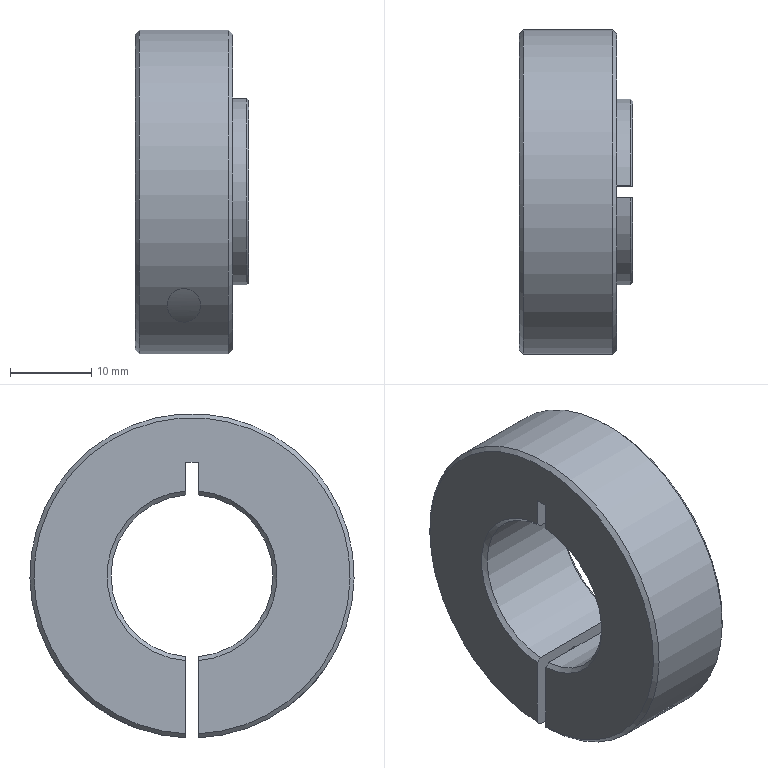Part | NX | features 1_11 2 | 1 solid | 28 faces | box 14 x 40 x 39.986 mm | volume 10434 mm3 | plane 10 | cone 9 | cylinder 9 | commonest cylinder face diameters 20 x2 23 x2 40 x2 4.134 x1 5.5 x1 9 x1
STEP:
#1=CARTESIAN_POINT('',(-123.,-261.55,-709.529));
#2=VERTEX_POINT('',#1);
#3=CARTESIAN_POINT('',(-125.5,-261.55,-709.529));
#4=DIRECTION('',(0.,-1.,0.));
#5=DIRECTION('',(1.,0.,0.));
#6=AXIS2_PLACEMENT_3D('',#3,#4,#5);
#7=CIRCLE('',#6,2.5);
#8=EDGE_CURVE('',#2,#2,#7,.T.);
#9=ORIENTED_EDGE('',*,*,#8,.F.);
#10=EDGE_LOOP('',(#9));
#11=FACE_BOUND('',#10,.T.);
#12=CARTESIAN_POINT('',(-127.567,-261.983,-709.529));
#13=VERTEX_POINT('',#12);
#14=CARTESIAN_POINT('',(-125.5,-261.983,-709.529));
#15=DIRECTION('',(0.,-1.,0.));
#16=DIRECTION('',(-1.,0.,0.));
#17=AXIS2_PLACEMENT_3D('',#14,#15,#16);
#18=CIRCLE('',#17,2.067);
#19=EDGE_CURVE('',#13,#13,#18,.T.);
#20=ORIENTED_EDGE('',*,*,#19,.T.);
#21=EDGE_LOOP('',(#20));
#22=FACE_BOUND('',#21,.T.);
#23=CARTESIAN_POINT('',(-125.5,-262.032,-709.529));
#24=DIRECTION('',(0.,1.,0.));
#25=DIRECTION('',(-1.,0.,0.));
#26=AXIS2_PLACEMENT_3D('',#23,#24,#25);
#27=CONICAL_SURFACE('',#26,2.018,0.7854);
#28=ADVANCED_FACE('',(#11,#22),#27,.F.);
#29=CARTESIAN_POINT('',(-127.567,-275.083,-709.529));
#30=VERTEX_POINT('',#29);
#31=CARTESIAN_POINT('',(-123.433,-275.083,-709.529));
#32=VERTEX_POINT('',#31);
#33=CARTESIAN_POINT('',(-123.433,-275.083,-709.529));
#34=CARTESIAN_POINT('',(-123.433,-274.603,-710.02));
#35=CARTESIAN_POINT('',(-123.683,-273.842,-710.714));
#36=CARTESIAN_POINT('',(-124.497,-272.96,-711.413));
#37=CARTESIAN_POINT('',(-125.5,-272.586,-711.688));
#38=CARTESIAN_POINT('',(-126.503,-272.96,-711.413));
#39=CARTESIAN_POINT('',(-127.317,-273.842,-710.714));
#40=CARTESIAN_POINT('',(-127.567,-274.603,-710.02));
#41=CARTESIAN_POINT('',(-127.567,-275.083,-709.529));
#42=B_SPLINE_CURVE_WITH_KNOTS('',3,(#33,#34,#35,#36,#37,#38,#39,#40,#41),.UNSPECIFIED.,.F.,.F.,(4,1,1,1,1,1,4),(0.,0.25,0.375,0.5,0.625,0.75,1.),.UNSPECIFIED.);
#43=EDGE_CURVE('',#30,#32,#42,.F.);
#44=ORIENTED_EDGE('',*,*,#43,.T.);
#45=CARTESIAN_POINT('',(-127.567,-275.083,-709.529));
#46=CARTESIAN_POINT('',(-127.567,-275.524,-709.078));
#47=CARTESIAN_POINT('',(-127.348,-276.166,-708.351));
#48=CARTESIAN_POINT('',(-126.445,-276.738,-707.615));
#49=CARTESIAN_POINT('',(-125.5,-276.906,-707.386));
#50=CARTESIAN_POINT('',(-124.555,-276.738,-707.615));
#51=CARTESIAN_POINT('',(-123.652,-276.166,-708.351));
#52=CARTESIAN_POINT('',(-123.433,-275.524,-709.078));
#53=CARTESIAN_POINT('',(-123.433,-275.083,-709.529));
#54=B_SPLINE_CURVE_WITH_KNOTS('',3,(#45,#46,#47,#48,#49,#50,#51,#52,#53),.UNSPECIFIED.,.F.,.F.,(4,1,1,1,1,1,4),(0.,0.25,0.375,0.5,0.625,0.75,1.),.UNSPECIFIED.);
#55=EDGE_CURVE('',#32,#30,#54,.F.);
#56=ORIENTED_EDGE('',*,*,#55,.T.);
#57=EDGE_LOOP('',(#44,#56));
#58=FACE_BOUND('',#57,.T.);
#59=ORIENTED_EDGE('',*,*,#19,.F.);
#60=EDGE_LOOP('',(#59));
#61=FACE_BOUND('',#60,.T.);
#62=CARTESIAN_POINT('',(-125.5,-272.267,-709.529));
#63=DIRECTION('',(0.,-1.,0.));
#64=DIRECTION('',(1.,0.,0.));
#65=AXIS2_PLACEMENT_3D('',#62,#63,#64);
#66=CYLINDRICAL_SURFACE('',#65,2.067);
#67=ADVANCED_FACE('',(#58,#61),#66,.F.);
#68=CARTESIAN_POINT('',(-131.5,-261.55,-681.529));
#69=VERTEX_POINT('',#68);
#70=CARTESIAN_POINT('',(-131.5,-260.05,-681.529));
#71=VERTEX_POINT('',#70);
#72=CARTESIAN_POINT('',(-131.5,-261.55,-681.529));
#73=DIRECTION('',(0.,1.,0.));
#74=VECTOR('',#73,1000.);
#75=LINE('',#72,#74);
#76=EDGE_CURVE('',#69,#71,#75,.T.);
#77=ORIENTED_EDGE('',*,*,#76,.T.);
#78=CARTESIAN_POINT('',(-119.5,-260.05,-681.529));
#79=VERTEX_POINT('',#78);
#80=CARTESIAN_POINT('',(-119.5,-260.05,-681.529));
#81=DIRECTION('',(-1.,0.,0.));
#82=VECTOR('',#81,1000.);
#83=LINE('',#80,#82);
#84=EDGE_CURVE('',#79,#71,#83,.T.);
#85=ORIENTED_EDGE('',*,*,#84,.F.);
#86=CARTESIAN_POINT('',(-119.5,-261.55,-681.529));
#87=VERTEX_POINT('',#86);
#88=CARTESIAN_POINT('',(-119.5,-260.05,-681.529));
#89=DIRECTION('',(0.,-1.,0.));
#90=VECTOR('',#89,1000.);
#91=LINE('',#88,#90);
#92=EDGE_CURVE('',#79,#87,#91,.T.);
#93=ORIENTED_EDGE('',*,*,#92,.T.);
#94=CARTESIAN_POINT('',(-131.5,-261.55,-681.529));
#95=DIRECTION('',(1.,0.,0.));
#96=VECTOR('',#95,1000.);
#97=LINE('',#94,#96);
#98=EDGE_CURVE('',#69,#87,#97,.T.);
#99=ORIENTED_EDGE('',*,*,#98,.F.);
#100=EDGE_LOOP('',(#77,#85,#93,#99));
#101=FACE_BOUND('',#100,.T.);
#102=CARTESIAN_POINT('',(-149.5,-261.55,-681.529));
#103=DIRECTION('',(0.,0.,1.));
#104=DIRECTION('',(0.,1.,0.));
#105=AXIS2_PLACEMENT_3D('',#102,#103,#104);
#106=PLANE('',#105);
#107=ADVANCED_FACE('',(#101),#106,.F.);
#108=CARTESIAN_POINT('',(-131.5,-260.05,-685.056));
#109=VERTEX_POINT('',#108);
#110=CARTESIAN_POINT('',(-131.5,-260.05,-681.529));
#111=DIRECTION('',(0.,0.,-1.));
#112=VECTOR('',#111,1000.);
#113=LINE('',#110,#112);
#114=EDGE_CURVE('',#71,#109,#113,.T.);
#115=ORIENTED_EDGE('',*,*,#114,.T.);
#116=CARTESIAN_POINT('',(-131.,-260.05,-685.558));
#117=VERTEX_POINT('',#116);
#118=CARTESIAN_POINT('',(-131.5,-260.05,-685.056));
#119=CARTESIAN_POINT('',(-131.333,-260.05,-685.223));
#120=CARTESIAN_POINT('',(-131.167,-260.05,-685.39));
#121=CARTESIAN_POINT('',(-131.,-260.05,-685.558));
#122=B_SPLINE_CURVE_WITH_KNOTS('',3,(#118,#119,#120,#121),.UNSPECIFIED.,.F.,.F.,(4,4),(0.,1.),.UNSPECIFIED.);
#123=EDGE_CURVE('',#117,#109,#122,.F.);
#124=ORIENTED_EDGE('',*,*,#123,.F.);
#125=CARTESIAN_POINT('',(-118.,-260.05,-685.558));
#126=VERTEX_POINT('',#125);
#127=CARTESIAN_POINT('',(-118.,-260.05,-685.558));
#128=DIRECTION('',(-1.,0.,0.));
#129=VECTOR('',#128,1000.);
#130=LINE('',#127,#129);
#131=EDGE_CURVE('',#126,#117,#130,.T.);
#132=ORIENTED_EDGE('',*,*,#131,.F.);
#133=CARTESIAN_POINT('',(-117.5,-260.05,-685.056));
#134=VERTEX_POINT('',#133);
#135=CARTESIAN_POINT('',(-118.,-260.05,-685.558));
#136=CARTESIAN_POINT('',(-117.833,-260.05,-685.39));
#137=CARTESIAN_POINT('',(-117.667,-260.05,-685.223));
#138=CARTESIAN_POINT('',(-117.5,-260.05,-685.056));
#139=B_SPLINE_CURVE_WITH_KNOTS('',3,(#135,#136,#137,#138),.UNSPECIFIED.,.F.,.F.,(4,4),(0.,1.),.UNSPECIFIED.);
#140=EDGE_CURVE('',#134,#126,#139,.F.);
#141=ORIENTED_EDGE('',*,*,#140,.F.);
#142=CARTESIAN_POINT('',(-117.5,-260.05,-684.279));
#143=VERTEX_POINT('',#142);
#144=CARTESIAN_POINT('',(-117.5,-260.05,-685.056));
#145=DIRECTION('',(0.,0.,1.));
#146=VECTOR('',#145,1000.);
#147=LINE('',#144,#146);
#148=EDGE_CURVE('',#134,#143,#147,.T.);
#149=ORIENTED_EDGE('',*,*,#148,.T.);
#150=CARTESIAN_POINT('',(-117.725,-260.05,-684.054));
#151=VERTEX_POINT('',#150);
#152=CARTESIAN_POINT('',(-117.5,-260.05,-684.279));
#153=CARTESIAN_POINT('',(-117.575,-260.05,-684.204));
#154=CARTESIAN_POINT('',(-117.65,-260.05,-684.129));
#155=CARTESIAN_POINT('',(-117.725,-260.05,-684.054));
#156=B_SPLINE_CURVE_WITH_KNOTS('',3,(#152,#153,#154,#155),.UNSPECIFIED.,.F.,.F.,(4,4),(0.,1.),.UNSPECIFIED.);
#157=EDGE_CURVE('',#151,#143,#156,.F.);
#158=ORIENTED_EDGE('',*,*,#157,.F.);
#159=CARTESIAN_POINT('',(-119.5,-260.05,-684.054));
#160=VERTEX_POINT('',#159);
#161=CARTESIAN_POINT('',(-119.5,-260.05,-684.054));
#162=DIRECTION('',(1.,0.,0.));
#163=VECTOR('',#162,1000.);
#164=LINE('',#161,#163);
#165=EDGE_CURVE('',#160,#151,#164,.T.);
#166=ORIENTED_EDGE('',*,*,#165,.F.);
#167=CARTESIAN_POINT('',(-119.5,-260.05,-684.054));
#168=DIRECTION('',(0.,0.,1.));
#169=VECTOR('',#168,1000.);
#170=LINE('',#167,#169);
#171=EDGE_CURVE('',#160,#79,#170,.T.);
#172=ORIENTED_EDGE('',*,*,#171,.T.);
#173=ORIENTED_EDGE('',*,*,#84,.T.);
#174=EDGE_LOOP('',(#115,#124,#132,#141,#149,#158,#166,#172,#173));
#175=FACE_BOUND('',#174,.T.);
#176=CARTESIAN_POINT('',(-149.5,-260.05,-681.529));
#177=DIRECTION('',(0.,1.,0.));
#178=DIRECTION('',(-1.,0.,0.));
#179=AXIS2_PLACEMENT_3D('',#176,#177,#178);
#180=PLANE('',#179);
#181=ADVANCED_FACE('',(#175),#180,.F.);
#182=CARTESIAN_POINT('',(-131.,-260.05,-705.501));
#183=VERTEX_POINT('',#182);
#184=CARTESIAN_POINT('',(-131.,-260.8,-695.529));
#185=DIRECTION('',(1.,0.,0.));
#186=DIRECTION('',(0.,1.,0.));
#187=AXIS2_PLACEMENT_3D('',#184,#185,#186);
#188=CIRCLE('',#187,10.);
#189=EDGE_CURVE('',#183,#117,#188,.T.);
#190=ORIENTED_EDGE('',*,*,#189,.F.);
#191=CARTESIAN_POINT('',(-118.,-260.05,-705.501));
#192=VERTEX_POINT('',#191);
#193=CARTESIAN_POINT('',(-131.,-260.05,-705.501));
#194=DIRECTION('',(1.,0.,0.));
#195=VECTOR('',#194,1000.);
#196=LINE('',#193,#195);
#197=EDGE_CURVE('',#183,#192,#196,.T.);
#198=ORIENTED_EDGE('',*,*,#197,.T.);
#199=CARTESIAN_POINT('',(-118.,-260.8,-695.529));
#200=DIRECTION('',(-1.,0.,0.));
#201=DIRECTION('',(0.,1.,0.));
#202=AXIS2_PLACEMENT_3D('',#199,#200,#201);
#203=CIRCLE('',#202,10.);
#204=EDGE_CURVE('',#126,#192,#203,.T.);
#205=ORIENTED_EDGE('',*,*,#204,.F.);
#206=ORIENTED_EDGE('',*,*,#131,.T.);
#207=EDGE_LOOP('',(#190,#198,#205,#206));
#208=FACE_BOUND('',#207,.T.);
#209=CARTESIAN_POINT('',(-124.5,-260.8,-695.529));
#210=DIRECTION('',(-1.,0.,0.));
#211=DIRECTION('',(0.,-1.,0.));
#212=AXIS2_PLACEMENT_3D('',#209,#210,#211);
#213=CYLINDRICAL_SURFACE('',#212,10.);
#214=ADVANCED_FACE('',(#208),#213,.F.);
#215=ORIENTED_EDGE('',*,*,#204,.T.);
#216=CARTESIAN_POINT('',(-117.5,-260.05,-706.003));
#217=VERTEX_POINT('',#216);
#218=CARTESIAN_POINT('',(-117.5,-260.05,-706.003));
#219=CARTESIAN_POINT('',(-117.667,-260.05,-705.835));
#220=CARTESIAN_POINT('',(-117.833,-260.05,-705.668));
#221=CARTESIAN_POINT('',(-118.,-260.05,-705.501));
#222=B_SPLINE_CURVE_WITH_KNOTS('',3,(#218,#219,#220,#221),.UNSPECIFIED.,.F.,.F.,(4,4),(0.,1.),.UNSPECIFIED.);
#223=EDGE_CURVE('',#192,#217,#222,.F.);
#224=ORIENTED_EDGE('',*,*,#223,.T.);
#225=CARTESIAN_POINT('',(-117.5,-260.8,-695.529));
#226=DIRECTION('',(-1.,0.,0.));
#227=DIRECTION('',(0.,1.,0.));
#228=AXIS2_PLACEMENT_3D('',#225,#226,#227);
#229=CIRCLE('',#228,10.5);
#230=EDGE_CURVE('',#134,#217,#229,.T.);
#231=ORIENTED_EDGE('',*,*,#230,.F.);
#232=ORIENTED_EDGE('',*,*,#140,.T.);
#233=EDGE_LOOP('',(#215,#224,#231,#232));
#234=FACE_BOUND('',#233,.T.);
#235=CARTESIAN_POINT('',(-118.049,-260.8,-695.529));
#236=DIRECTION('',(1.,0.,0.));
#237=DIRECTION('',(0.,1.,0.));
#238=AXIS2_PLACEMENT_3D('',#235,#236,#237);
#239=CONICAL_SURFACE('',#238,9.951,0.7854);
#240=ADVANCED_FACE('',(#234),#239,.F.);
#241=CARTESIAN_POINT('',(-117.5,-260.05,-706.779));
#242=VERTEX_POINT('',#241);
#243=CARTESIAN_POINT('',(-117.5,-260.8,-695.529));
#244=DIRECTION('',(1.,0.,0.));
#245=DIRECTION('',(0.,0.06652,-0.9978));
#246=AXIS2_PLACEMENT_3D('',#243,#244,#245);
#247=CIRCLE('',#246,11.275);
#248=EDGE_CURVE('',#242,#143,#247,.T.);
#249=ORIENTED_EDGE('',*,*,#248,.T.);
#250=ORIENTED_EDGE('',*,*,#148,.F.);
#251=ORIENTED_EDGE('',*,*,#230,.T.);
#252=CARTESIAN_POINT('',(-117.5,-260.05,-706.779));
#253=DIRECTION('',(0.,0.,1.));
#254=VECTOR('',#253,1000.);
#255=LINE('',#252,#254);
#256=EDGE_CURVE('',#242,#217,#255,.T.);
#257=ORIENTED_EDGE('',*,*,#256,.F.);
#258=EDGE_LOOP('',(#249,#250,#251,#257));
#259=FACE_BOUND('',#258,.T.);
#260=CARTESIAN_POINT('',(-117.5,-260.8,-684.642));
#261=DIRECTION('',(1.,0.,0.));
#262=DIRECTION('',(0.,1.,0.));
#263=AXIS2_PLACEMENT_3D('',#260,#261,#262);
#264=PLANE('',#263);
#265=ADVANCED_FACE('',(#259),#264,.T.);
#266=CARTESIAN_POINT('',(-117.725,-260.05,-707.005));
#267=VERTEX_POINT('',#266);
#268=CARTESIAN_POINT('',(-117.725,-260.8,-695.529));
#269=DIRECTION('',(1.,0.,0.));
#270=DIRECTION('',(0.,0.06522,-0.9979));
#271=AXIS2_PLACEMENT_3D('',#268,#269,#270);
#272=CIRCLE('',#271,11.5);
#273=EDGE_CURVE('',#267,#151,#272,.T.);
#274=ORIENTED_EDGE('',*,*,#273,.T.);
#275=ORIENTED_EDGE('',*,*,#157,.T.);
#276=ORIENTED_EDGE('',*,*,#248,.F.);
#277=CARTESIAN_POINT('',(-117.725,-260.05,-707.005));
#278=CARTESIAN_POINT('',(-117.65,-260.05,-706.93));
#279=CARTESIAN_POINT('',(-117.575,-260.05,-706.855));
#280=CARTESIAN_POINT('',(-117.5,-260.05,-706.779));
#281=B_SPLINE_CURVE_WITH_KNOTS('',3,(#277,#278,#279,#280),.UNSPECIFIED.,.F.,.F.,(4,4),(0.,1.),.UNSPECIFIED.);
#282=EDGE_CURVE('',#242,#267,#281,.F.);
#283=ORIENTED_EDGE('',*,*,#282,.T.);
#284=EDGE_LOOP('',(#274,#275,#276,#283));
#285=FACE_BOUND('',#284,.T.);
#286=CARTESIAN_POINT('',(-117.451,-260.8,-695.529));
#287=DIRECTION('',(-1.,0.,0.));
#288=DIRECTION('',(0.,-1.,0.));
#289=AXIS2_PLACEMENT_3D('',#286,#287,#288);
#290=CONICAL_SURFACE('',#289,11.226,0.7854);
#291=ADVANCED_FACE('',(#285),#290,.T.);
#292=CARTESIAN_POINT('',(-119.5,-260.05,-707.005));
#293=VERTEX_POINT('',#292);
#294=CARTESIAN_POINT('',(-119.5,-260.8,-695.529));
#295=DIRECTION('',(-1.,0.,0.));
#296=DIRECTION('',(0.,1.,0.));
#297=AXIS2_PLACEMENT_3D('',#294,#295,#296);
#298=CIRCLE('',#297,11.5);
#299=EDGE_CURVE('',#160,#293,#298,.T.);
#300=ORIENTED_EDGE('',*,*,#299,.F.);
#301=ORIENTED_EDGE('',*,*,#165,.T.);
#302=ORIENTED_EDGE('',*,*,#273,.F.);
#303=CARTESIAN_POINT('',(-117.725,-260.05,-707.005));
#304=DIRECTION('',(-1.,0.,0.));
#305=VECTOR('',#304,1000.);
#306=LINE('',#303,#305);
#307=EDGE_CURVE('',#267,#293,#306,.T.);
#308=ORIENTED_EDGE('',*,*,#307,.T.);
#309=EDGE_LOOP('',(#300,#301,#302,#308));
#310=FACE_BOUND('',#309,.T.);
#311=CARTESIAN_POINT('',(-118.612,-260.8,-695.529));
#312=DIRECTION('',(-1.,0.,0.));
#313=DIRECTION('',(0.,-1.,0.));
#314=AXIS2_PLACEMENT_3D('',#311,#312,#313);
#315=CYLINDRICAL_SURFACE('',#314,11.5);
#316=ADVANCED_FACE('',(#310),#315,.T.);
#317=CARTESIAN_POINT('',(-119.5,-260.05,-715.015));
#318=VERTEX_POINT('',#317);
#319=CARTESIAN_POINT('',(-119.5,-260.05,-715.015));
#320=DIRECTION('',(0.,0.,1.));
#321=VECTOR('',#320,1000.);
#322=LINE('',#319,#321);
#323=EDGE_CURVE('',#318,#293,#322,.T.);
#324=ORIENTED_EDGE('',*,*,#323,.F.);
#325=CARTESIAN_POINT('',(-119.5,-261.55,-715.015));
#326=VERTEX_POINT('',#325);
#327=CARTESIAN_POINT('',(-119.5,-260.8,-695.529));
#328=DIRECTION('',(1.,0.,0.));
#329=DIRECTION('',(0.,1.,0.));
#330=AXIS2_PLACEMENT_3D('',#327,#328,#329);
#331=CIRCLE('',#330,19.5);
#332=EDGE_CURVE('',#318,#326,#331,.T.);
#333=ORIENTED_EDGE('',*,*,#332,.T.);
#334=CARTESIAN_POINT('',(-119.5,-261.55,-707.005));
#335=VERTEX_POINT('',#334);
#336=CARTESIAN_POINT('',(-119.5,-261.55,-707.005));
#337=DIRECTION('',(0.,0.,-1.));
#338=VECTOR('',#337,1000.);
#339=LINE('',#336,#338);
#340=EDGE_CURVE('',#335,#326,#339,.T.);
#341=ORIENTED_EDGE('',*,*,#340,.F.);
#342=CARTESIAN_POINT('',(-119.5,-261.55,-684.054));
#343=VERTEX_POINT('',#342);
#344=CARTESIAN_POINT('',(-119.5,-260.8,-695.529));
#345=DIRECTION('',(-1.,0.,0.));
#346=DIRECTION('',(0.,-1.,0.));
#347=AXIS2_PLACEMENT_3D('',#344,#345,#346);
#348=CIRCLE('',#347,11.5);
#349=EDGE_CURVE('',#335,#343,#348,.T.);
#350=ORIENTED_EDGE('',*,*,#349,.T.);
#351=CARTESIAN_POINT('',(-119.5,-261.55,-681.529));
#352=DIRECTION('',(0.,0.,-1.));
#353=VECTOR('',#352,1000.);
#354=LINE('',#351,#353);
#355=EDGE_CURVE('',#87,#343,#354,.T.);
#356=ORIENTED_EDGE('',*,*,#355,.F.);
#357=ORIENTED_EDGE('',*,*,#92,.F.);
#358=ORIENTED_EDGE('',*,*,#171,.F.);
#359=ORIENTED_EDGE('',*,*,#299,.T.);
#360=EDGE_LOOP('',(#324,#333,#341,#350,#356,#357,#358,#359));
#361=FACE_BOUND('',#360,.T.);
#362=CARTESIAN_POINT('',(-119.5,-260.8,-680.029));
#363=DIRECTION('',(1.,0.,0.));
#364=DIRECTION('',(0.,1.,0.));
#365=AXIS2_PLACEMENT_3D('',#362,#363,#364);
#366=PLANE('',#365);
#367=ADVANCED_FACE('',(#361),#366,.T.);
#368=ORIENTED_EDGE('',*,*,#332,.F.);
#369=CARTESIAN_POINT('',(-120.,-260.05,-715.515));
#370=VERTEX_POINT('',#369);
#371=CARTESIAN_POINT('',(-120.,-260.05,-715.515));
#372=CARTESIAN_POINT('',(-119.833,-260.05,-715.349));
#373=CARTESIAN_POINT('',(-119.667,-260.05,-715.182));
#374=CARTESIAN_POINT('',(-119.5,-260.05,-715.015));
#375=B_SPLINE_CURVE_WITH_KNOTS('',3,(#371,#372,#373,#374),.UNSPECIFIED.,.F.,.F.,(4,4),(0.,1.),.UNSPECIFIED.);
#376=EDGE_CURVE('',#318,#370,#375,.F.);
#377=ORIENTED_EDGE('',*,*,#376,.T.);
#378=CARTESIAN_POINT('',(-120.,-261.55,-715.515));
#379=VERTEX_POINT('',#378);
#380=CARTESIAN_POINT('',(-120.,-260.8,-695.529));
#381=DIRECTION('',(1.,0.,0.));
#382=DIRECTION('',(0.,0.0375,-0.9993));
#383=AXIS2_PLACEMENT_3D('',#380,#381,#382);
#384=CIRCLE('',#383,20.);
#385=EDGE_CURVE('',#370,#379,#384,.T.);
#386=ORIENTED_EDGE('',*,*,#385,.T.);
#387=CARTESIAN_POINT('',(-119.5,-261.55,-715.015));
#388=CARTESIAN_POINT('',(-119.667,-261.55,-715.182));
#389=CARTESIAN_POINT('',(-119.833,-261.55,-715.349));
#390=CARTESIAN_POINT('',(-120.,-261.55,-715.515));
#391=B_SPLINE_CURVE_WITH_KNOTS('',3,(#387,#388,#389,#390),.UNSPECIFIED.,.F.,.F.,(4,4),(0.,1.),.UNSPECIFIED.);
#392=EDGE_CURVE('',#379,#326,#391,.F.);
#393=ORIENTED_EDGE('',*,*,#392,.T.);
#394=EDGE_LOOP('',(#368,#377,#386,#393));
#395=FACE_BOUND('',#394,.T.);
#396=CARTESIAN_POINT('',(-119.451,-260.8,-695.529));
#397=DIRECTION('',(-1.,0.,0.));
#398=DIRECTION('',(0.,-1.,0.));
#399=AXIS2_PLACEMENT_3D('',#396,#397,#398);
#400=CONICAL_SURFACE('',#399,19.451,0.7854);
#401=ADVANCED_FACE('',(#395),#400,.T.);
#402=CARTESIAN_POINT('',(-130.,-246.517,-709.529));
#403=VERTEX_POINT('',#402);
#404=CARTESIAN_POINT('',(-121.,-246.517,-709.529));
#405=VERTEX_POINT('',#404);
#406=CARTESIAN_POINT('',(-130.,-246.517,-709.529));
#407=CARTESIAN_POINT('',(-130.,-245.584,-708.578));
#408=CARTESIAN_POINT('',(-129.528,-244.31,-706.94));
#409=CARTESIAN_POINT('',(-127.503,-243.362,-705.337));
#410=CARTESIAN_POINT('',(-125.5,-243.119,-704.875));
#411=CARTESIAN_POINT('',(-123.497,-243.362,-705.337));
#412=CARTESIAN_POINT('',(-121.472,-244.31,-706.941));
#413=CARTESIAN_POINT('',(-121.,-245.584,-708.578));
#414=CARTESIAN_POINT('',(-121.,-246.517,-709.529));
#415=B_SPLINE_CURVE_WITH_KNOTS('',3,(#406,#407,#408,#409,#410,#411,#412,#413,#414),.UNSPECIFIED.,.F.,.F.,(4,1,1,1,1,1,4),(0.,0.25,0.375,0.5,0.625,0.75,1.),.UNSPECIFIED.);
#416=EDGE_CURVE('',#403,#405,#415,.T.);
#417=ORIENTED_EDGE('',*,*,#416,.F.);
#418=CARTESIAN_POINT('',(-121.,-246.517,-709.529));
#419=CARTESIAN_POINT('',(-121.001,-247.096,-710.12));
#420=CARTESIAN_POINT('',(-121.228,-248.323,-711.223));
#421=CARTESIAN_POINT('',(-122.061,-250.246,-712.569));
#422=CARTESIAN_POINT('',(-123.116,-251.825,-713.423));
#423=CARTESIAN_POINT('',(-124.285,-252.902,-713.909));
#424=CARTESIAN_POINT('',(-125.5,-253.347,-714.089));
#425=CARTESIAN_POINT('',(-126.716,-252.903,-713.909));
#426=CARTESIAN_POINT('',(-127.884,-251.825,-713.423));
#427=CARTESIAN_POINT('',(-128.939,-250.246,-712.569));
#428=CARTESIAN_POINT('',(-129.772,-248.323,-711.223));
#429=CARTESIAN_POINT('',(-129.999,-247.096,-710.12));
#430=CARTESIAN_POINT('',(-130.,-246.517,-709.529));
#431=B_SPLINE_CURVE_WITH_KNOTS('',3,(#418,#419,#420,#421,#422,#423,#424,#425,#426,#427,#428,#429,#430),.UNSPECIFIED.,.F.,.F.,(4,1,1,1,1,1,1,1,1,1,4),(0.,0.125,0.25,0.375,0.4375,0.5,0.5625,0.625,0.75,0.875,1.),.UNSPECIFIED.);
#432=EDGE_CURVE('',#405,#403,#431,.T.);
#433=ORIENTED_EDGE('',*,*,#432,.F.);
#434=EDGE_LOOP('',(#417,#433));
#435=FACE_BOUND('',#434,.T.);
#436=ORIENTED_EDGE('',*,*,#385,.F.);
#437=CARTESIAN_POINT('',(-131.,-260.05,-715.515));
#438=VERTEX_POINT('',#437);
#439=CARTESIAN_POINT('',(-120.,-260.05,-715.515));
#440=DIRECTION('',(-1.,0.,0.));
#441=VECTOR('',#440,1000.);
#442=LINE('',#439,#441);
#443=EDGE_CURVE('',#370,#438,#442,.T.);
#444=ORIENTED_EDGE('',*,*,#443,.T.);
#445=CARTESIAN_POINT('',(-131.,-261.55,-715.515));
#446=VERTEX_POINT('',#445);
#447=CARTESIAN_POINT('',(-131.,-260.8,-695.529));
#448=DIRECTION('',(-1.,0.,0.));
#449=DIRECTION('',(0.,-0.0375,-0.9993));
#450=AXIS2_PLACEMENT_3D('',#447,#448,#449);
#451=CIRCLE('',#450,20.);
#452=EDGE_CURVE('',#446,#438,#451,.T.);
#453=ORIENTED_EDGE('',*,*,#452,.F.);
#454=CARTESIAN_POINT('',(-131.,-261.55,-715.515));
#455=DIRECTION('',(1.,0.,0.));
#456=VECTOR('',#455,1000.);
#457=LINE('',#454,#456);
#458=EDGE_CURVE('',#446,#379,#457,.T.);
#459=ORIENTED_EDGE('',*,*,#458,.T.);
#460=EDGE_LOOP('',(#436,#444,#453,#459));
#461=FACE_BOUND('',#460,.T.);
#462=ORIENTED_EDGE('',*,*,#55,.F.);
#463=ORIENTED_EDGE('',*,*,#43,.F.);
#464=EDGE_LOOP('',(#462,#463));
#465=FACE_BOUND('',#464,.T.);
#466=CARTESIAN_POINT('',(-125.5,-260.8,-695.529));
#467=DIRECTION('',(-1.,0.,0.));
#468=DIRECTION('',(0.,-1.,0.));
#469=AXIS2_PLACEMENT_3D('',#466,#467,#468);
#470=CYLINDRICAL_SURFACE('',#469,20.);
#471=ADVANCED_FACE('',(#435,#461,#465),#470,.T.);
#472=CARTESIAN_POINT('',(-131.5,-261.55,-715.015));
#473=VERTEX_POINT('',#472);
#474=CARTESIAN_POINT('',(-131.5,-260.05,-715.015));
#475=VERTEX_POINT('',#474);
#476=CARTESIAN_POINT('',(-131.5,-260.8,-695.529));
#477=DIRECTION('',(-1.,0.,0.));
#478=DIRECTION('',(0.,1.,0.));
#479=AXIS2_PLACEMENT_3D('',#476,#477,#478);
#480=CIRCLE('',#479,19.5);
#481=EDGE_CURVE('',#473,#475,#480,.T.);
#482=ORIENTED_EDGE('',*,*,#481,.F.);
#483=CARTESIAN_POINT('',(-131.,-261.55,-715.515));
#484=CARTESIAN_POINT('',(-131.167,-261.55,-715.349));
#485=CARTESIAN_POINT('',(-131.333,-261.55,-715.182));
#486=CARTESIAN_POINT('',(-131.5,-261.55,-715.015));
#487=B_SPLINE_CURVE_WITH_KNOTS('',3,(#483,#484,#485,#486),.UNSPECIFIED.,.F.,.F.,(4,4),(0.,1.),.UNSPECIFIED.);
#488=EDGE_CURVE('',#473,#446,#487,.F.);
#489=ORIENTED_EDGE('',*,*,#488,.T.);
#490=ORIENTED_EDGE('',*,*,#452,.T.);
#491=CARTESIAN_POINT('',(-131.5,-260.05,-715.015));
#492=CARTESIAN_POINT('',(-131.333,-260.05,-715.182));
#493=CARTESIAN_POINT('',(-131.167,-260.05,-715.349));
#494=CARTESIAN_POINT('',(-131.,-260.05,-715.515));
#495=B_SPLINE_CURVE_WITH_KNOTS('',3,(#491,#492,#493,#494),.UNSPECIFIED.,.F.,.F.,(4,4),(0.,1.),.UNSPECIFIED.);
#496=EDGE_CURVE('',#438,#475,#495,.F.);
#497=ORIENTED_EDGE('',*,*,#496,.T.);
#498=EDGE_LOOP('',(#482,#489,#490,#497));
#499=FACE_BOUND('',#498,.T.);
#500=CARTESIAN_POINT('',(-131.549,-260.8,-695.529));
#501=DIRECTION('',(1.,0.,0.));
#502=DIRECTION('',(0.,1.,0.));
#503=AXIS2_PLACEMENT_3D('',#500,#501,#502);
#504=CONICAL_SURFACE('',#503,19.451,0.7854);
#505=ADVANCED_FACE('',(#499),#504,.T.);
#506=ORIENTED_EDGE('',*,*,#8,.T.);
#507=EDGE_LOOP('',(#506));
#508=FACE_BOUND('',#507,.T.);
#509=CARTESIAN_POINT('',(-117.5,-261.55,-706.003));
#510=VERTEX_POINT('',#509);
#511=CARTESIAN_POINT('',(-117.5,-261.55,-706.779));
#512=VERTEX_POINT('',#511);
#513=CARTESIAN_POINT('',(-117.5,-261.55,-706.003));
#514=DIRECTION('',(0.,0.,-1.));
#515=VECTOR('',#514,1000.);
#516=LINE('',#513,#515);
#517=EDGE_CURVE('',#510,#512,#516,.T.);
#518=ORIENTED_EDGE('',*,*,#517,.T.);
#519=CARTESIAN_POINT('',(-117.725,-261.55,-707.005));
#520=VERTEX_POINT('',#519);
#521=CARTESIAN_POINT('',(-117.5,-261.55,-706.779));
#522=CARTESIAN_POINT('',(-117.575,-261.55,-706.855));
#523=CARTESIAN_POINT('',(-117.65,-261.55,-706.93));
#524=CARTESIAN_POINT('',(-117.725,-261.55,-707.005));
#525=B_SPLINE_CURVE_WITH_KNOTS('',3,(#521,#522,#523,#524),.UNSPECIFIED.,.F.,.F.,(4,4),(0.,1.),.UNSPECIFIED.);
#526=EDGE_CURVE('',#520,#512,#525,.F.);
#527=ORIENTED_EDGE('',*,*,#526,.F.);
#528=CARTESIAN_POINT('',(-119.5,-261.55,-707.005));
#529=DIRECTION('',(1.,0.,0.));
#530=VECTOR('',#529,1000.);
#531=LINE('',#528,#530);
#532=EDGE_CURVE('',#335,#520,#531,.T.);
#533=ORIENTED_EDGE('',*,*,#532,.F.);
#534=ORIENTED_EDGE('',*,*,#340,.T.);
#535=ORIENTED_EDGE('',*,*,#392,.F.);
#536=ORIENTED_EDGE('',*,*,#458,.F.);
#537=ORIENTED_EDGE('',*,*,#488,.F.);
#538=CARTESIAN_POINT('',(-131.5,-261.55,-706.003));
#539=VERTEX_POINT('',#538);
#540=CARTESIAN_POINT('',(-131.5,-261.55,-715.015));
#541=DIRECTION('',(0.,0.,1.));
#542=VECTOR('',#541,1000.);
#543=LINE('',#540,#542);
#544=EDGE_CURVE('',#473,#539,#543,.T.);
#545=ORIENTED_EDGE('',*,*,#544,.T.);
#546=CARTESIAN_POINT('',(-131.,-261.55,-705.501));
#547=VERTEX_POINT('',#546);
#548=CARTESIAN_POINT('',(-131.5,-261.55,-706.003));
#549=CARTESIAN_POINT('',(-131.333,-261.55,-705.835));
#550=CARTESIAN_POINT('',(-131.167,-261.55,-705.668));
#551=CARTESIAN_POINT('',(-131.,-261.55,-705.501));
#552=B_SPLINE_CURVE_WITH_KNOTS('',3,(#548,#549,#550,#551),.UNSPECIFIED.,.F.,.F.,(4,4),(0.,1.),.UNSPECIFIED.);
#553=EDGE_CURVE('',#547,#539,#552,.F.);
#554=ORIENTED_EDGE('',*,*,#553,.F.);
#555=CARTESIAN_POINT('',(-118.,-261.55,-705.501));
#556=VERTEX_POINT('',#555);
#557=CARTESIAN_POINT('',(-118.,-261.55,-705.501));
#558=DIRECTION('',(-1.,0.,0.));
#559=VECTOR('',#558,1000.);
#560=LINE('',#557,#559);
#561=EDGE_CURVE('',#556,#547,#560,.T.);
#562=ORIENTED_EDGE('',*,*,#561,.F.);
#563=CARTESIAN_POINT('',(-118.,-261.55,-705.501));
#564=CARTESIAN_POINT('',(-117.833,-261.55,-705.668));
#565=CARTESIAN_POINT('',(-117.667,-261.55,-705.835));
#566=CARTESIAN_POINT('',(-117.5,-261.55,-706.003));
#567=B_SPLINE_CURVE_WITH_KNOTS('',3,(#563,#564,#565,#566),.UNSPECIFIED.,.F.,.F.,(4,4),(0.,1.),.UNSPECIFIED.);
#568=EDGE_CURVE('',#510,#556,#567,.F.);
#569=ORIENTED_EDGE('',*,*,#568,.F.);
#570=EDGE_LOOP('',(#518,#527,#533,#534,#535,#536,#537,#545,#554,#562,#569));
#571=FACE_BOUND('',#570,.T.);
#572=CARTESIAN_POINT('',(-149.5,-261.55,-715.529));
#573=DIRECTION('',(0.,-1.,0.));
#574=DIRECTION('',(1.,0.,0.));
#575=AXIS2_PLACEMENT_3D('',#572,#573,#574);
#576=PLANE('',#575);
#577=ADVANCED_FACE('',(#508,#571),#576,.F.);
#578=CARTESIAN_POINT('',(-131.5,-261.55,-685.056));
#579=VERTEX_POINT('',#578);
#580=CARTESIAN_POINT('',(-131.,-261.55,-685.558));
#581=VERTEX_POINT('',#580);
#582=CARTESIAN_POINT('',(-131.,-261.55,-685.558));
#583=CARTESIAN_POINT('',(-131.167,-261.55,-685.39));
#584=CARTESIAN_POINT('',(-131.333,-261.55,-685.223));
#585=CARTESIAN_POINT('',(-131.5,-261.55,-685.056));
#586=B_SPLINE_CURVE_WITH_KNOTS('',3,(#582,#583,#584,#585),.UNSPECIFIED.,.F.,.F.,(4,4),(0.,1.),.UNSPECIFIED.);
#587=EDGE_CURVE('',#579,#581,#586,.F.);
#588=ORIENTED_EDGE('',*,*,#587,.T.);
#589=CARTESIAN_POINT('',(-131.,-260.8,-695.529));
#590=DIRECTION('',(1.,0.,0.));
#591=DIRECTION('',(0.,-1.,0.));
#592=AXIS2_PLACEMENT_3D('',#589,#590,#591);
#593=CIRCLE('',#592,10.);
#594=EDGE_CURVE('',#581,#547,#593,.T.);
#595=ORIENTED_EDGE('',*,*,#594,.T.);
#596=ORIENTED_EDGE('',*,*,#553,.T.);
#597=CARTESIAN_POINT('',(-131.5,-260.8,-695.529));
#598=DIRECTION('',(1.,0.,0.));
#599=DIRECTION('',(0.,-1.,0.));
#600=AXIS2_PLACEMENT_3D('',#597,#598,#599);
#601=CIRCLE('',#600,10.5);
#602=EDGE_CURVE('',#579,#539,#601,.T.);
#603=ORIENTED_EDGE('',*,*,#602,.F.);
#604=EDGE_LOOP('',(#588,#595,#596,#603));
#605=FACE_BOUND('',#604,.T.);
#606=CARTESIAN_POINT('',(-130.951,-260.8,-695.529));
#607=DIRECTION('',(-1.,0.,0.));
#608=DIRECTION('',(0.,-1.,0.));
#609=AXIS2_PLACEMENT_3D('',#606,#607,#608);
#610=CONICAL_SURFACE('',#609,9.951,0.7854);
#611=ADVANCED_FACE('',(#605),#610,.F.);
#612=CARTESIAN_POINT('',(-118.,-261.55,-685.558));
#613=VERTEX_POINT('',#612);
#614=CARTESIAN_POINT('',(-118.,-260.8,-695.529));
#615=DIRECTION('',(-1.,0.,0.));
#616=DIRECTION('',(0.,-0.075,-0.9972));
#617=AXIS2_PLACEMENT_3D('',#614,#615,#616);
#618=CIRCLE('',#617,10.);
#619=EDGE_CURVE('',#556,#613,#618,.T.);
#620=ORIENTED_EDGE('',*,*,#619,.F.);
#621=ORIENTED_EDGE('',*,*,#561,.T.);
#622=ORIENTED_EDGE('',*,*,#594,.F.);
#623=CARTESIAN_POINT('',(-131.,-261.55,-685.558));
#624=DIRECTION('',(1.,0.,0.));
#625=VECTOR('',#624,1000.);
#626=LINE('',#623,#625);
#627=EDGE_CURVE('',#581,#613,#626,.T.);
#628=ORIENTED_EDGE('',*,*,#627,.T.);
#629=EDGE_LOOP('',(#620,#621,#622,#628));
#630=FACE_BOUND('',#629,.T.);
#631=CARTESIAN_POINT('',(-124.5,-260.8,-695.529));
#632=DIRECTION('',(-1.,0.,0.));
#633=DIRECTION('',(0.,-1.,0.));
#634=AXIS2_PLACEMENT_3D('',#631,#632,#633);
#635=CYLINDRICAL_SURFACE('',#634,10.);
#636=ADVANCED_FACE('',(#630),#635,.F.);
#637=ORIENTED_EDGE('',*,*,#619,.T.);
#638=CARTESIAN_POINT('',(-117.5,-261.55,-685.056));
#639=VERTEX_POINT('',#638);
#640=CARTESIAN_POINT('',(-117.5,-261.55,-685.056));
#641=CARTESIAN_POINT('',(-117.667,-261.55,-685.223));
#642=CARTESIAN_POINT('',(-117.833,-261.55,-685.39));
#643=CARTESIAN_POINT('',(-118.,-261.55,-685.558));
#644=B_SPLINE_CURVE_WITH_KNOTS('',3,(#640,#641,#642,#643),.UNSPECIFIED.,.F.,.F.,(4,4),(0.,1.),.UNSPECIFIED.);
#645=EDGE_CURVE('',#613,#639,#644,.F.);
#646=ORIENTED_EDGE('',*,*,#645,.T.);
#647=CARTESIAN_POINT('',(-117.5,-260.8,-695.529));
#648=DIRECTION('',(-1.,0.,0.));
#649=DIRECTION('',(0.,-1.,0.));
#650=AXIS2_PLACEMENT_3D('',#647,#648,#649);
#651=CIRCLE('',#650,10.5);
#652=EDGE_CURVE('',#510,#639,#651,.T.);
#653=ORIENTED_EDGE('',*,*,#652,.F.);
#654=ORIENTED_EDGE('',*,*,#568,.T.);
#655=EDGE_LOOP('',(#637,#646,#653,#654));
#656=FACE_BOUND('',#655,.T.);
#657=CARTESIAN_POINT('',(-118.049,-260.8,-695.529));
#658=DIRECTION('',(1.,0.,0.));
#659=DIRECTION('',(0.,1.,0.));
#660=AXIS2_PLACEMENT_3D('',#657,#658,#659);
#661=CONICAL_SURFACE('',#660,9.951,0.7854);
#662=ADVANCED_FACE('',(#656),#661,.F.);
#663=CARTESIAN_POINT('',(-117.5,-261.55,-684.279));
#664=VERTEX_POINT('',#663);
#665=CARTESIAN_POINT('',(-117.5,-261.55,-684.279));
#666=DIRECTION('',(0.,0.,-1.));
#667=VECTOR('',#666,1000.);
#668=LINE('',#665,#667);
#669=EDGE_CURVE('',#664,#639,#668,.T.);
#670=ORIENTED_EDGE('',*,*,#669,.F.);
#671=CARTESIAN_POINT('',(-117.5,-260.8,-695.529));
#672=DIRECTION('',(1.,0.,0.));
#673=DIRECTION('',(0.,-1.,0.));
#674=AXIS2_PLACEMENT_3D('',#671,#672,#673);
#675=CIRCLE('',#674,11.275);
#676=EDGE_CURVE('',#664,#512,#675,.T.);
#677=ORIENTED_EDGE('',*,*,#676,.T.);
#678=ORIENTED_EDGE('',*,*,#517,.F.);
#679=ORIENTED_EDGE('',*,*,#652,.T.);
#680=EDGE_LOOP('',(#670,#677,#678,#679));
#681=FACE_BOUND('',#680,.T.);
#682=CARTESIAN_POINT('',(-117.5,-260.8,-684.642));
#683=DIRECTION('',(1.,0.,0.));
#684=DIRECTION('',(0.,1.,0.));
#685=AXIS2_PLACEMENT_3D('',#682,#683,#684);
#686=PLANE('',#685);
#687=ADVANCED_FACE('',(#681),#686,.T.);
#688=ORIENTED_EDGE('',*,*,#676,.F.);
#689=CARTESIAN_POINT('',(-117.725,-261.55,-684.054));
#690=VERTEX_POINT('',#689);
#691=CARTESIAN_POINT('',(-117.725,-261.55,-684.054));
#692=CARTESIAN_POINT('',(-117.65,-261.55,-684.129));
#693=CARTESIAN_POINT('',(-117.575,-261.55,-684.204));
#694=CARTESIAN_POINT('',(-117.5,-261.55,-684.279));
#695=B_SPLINE_CURVE_WITH_KNOTS('',3,(#691,#692,#693,#694),.UNSPECIFIED.,.F.,.F.,(4,4),(0.,1.),.UNSPECIFIED.);
#696=EDGE_CURVE('',#664,#690,#695,.F.);
#697=ORIENTED_EDGE('',*,*,#696,.T.);
#698=CARTESIAN_POINT('',(-117.725,-260.8,-695.529));
#699=DIRECTION('',(1.,0.,0.));
#700=DIRECTION('',(0.,-0.06522,0.9979));
#701=AXIS2_PLACEMENT_3D('',#698,#699,#700);
#702=CIRCLE('',#701,11.5);
#703=EDGE_CURVE('',#690,#520,#702,.T.);
#704=ORIENTED_EDGE('',*,*,#703,.T.);
#705=ORIENTED_EDGE('',*,*,#526,.T.);
#706=EDGE_LOOP('',(#688,#697,#704,#705));
#707=FACE_BOUND('',#706,.T.);
#708=CARTESIAN_POINT('',(-117.451,-260.8,-695.529));
#709=DIRECTION('',(-1.,0.,0.));
#710=DIRECTION('',(0.,-1.,0.));
#711=AXIS2_PLACEMENT_3D('',#708,#709,#710);
#712=CONICAL_SURFACE('',#711,11.226,0.7854);
#713=ADVANCED_FACE('',(#707),#712,.T.);
#714=ORIENTED_EDGE('',*,*,#703,.F.);
#715=CARTESIAN_POINT('',(-117.725,-261.55,-684.054));
#716=DIRECTION('',(-1.,0.,0.));
#717=VECTOR('',#716,1000.);
#718=LINE('',#715,#717);
#719=EDGE_CURVE('',#690,#343,#718,.T.);
#720=ORIENTED_EDGE('',*,*,#719,.T.);
#721=ORIENTED_EDGE('',*,*,#349,.F.);
#722=ORIENTED_EDGE('',*,*,#532,.T.);
#723=EDGE_LOOP('',(#714,#720,#721,#722));
#724=FACE_BOUND('',#723,.T.);
#725=CARTESIAN_POINT('',(-118.612,-260.8,-695.529));
#726=DIRECTION('',(-1.,0.,0.));
#727=DIRECTION('',(0.,-1.,0.));
#728=AXIS2_PLACEMENT_3D('',#725,#726,#727);
#729=CYLINDRICAL_SURFACE('',#728,11.5);
#730=ADVANCED_FACE('',(#724),#729,.T.);
#731=ORIENTED_EDGE('',*,*,#696,.F.);
#732=ORIENTED_EDGE('',*,*,#669,.T.);
#733=ORIENTED_EDGE('',*,*,#645,.F.);
#734=ORIENTED_EDGE('',*,*,#627,.F.);
#735=ORIENTED_EDGE('',*,*,#587,.F.);
#736=CARTESIAN_POINT('',(-131.5,-261.55,-685.056));
#737=DIRECTION('',(0.,0.,1.));
#738=VECTOR('',#737,1000.);
#739=LINE('',#736,#738);
#740=EDGE_CURVE('',#579,#69,#739,.T.);
#741=ORIENTED_EDGE('',*,*,#740,.T.);
#742=ORIENTED_EDGE('',*,*,#98,.T.);
#743=ORIENTED_EDGE('',*,*,#355,.T.);
#744=ORIENTED_EDGE('',*,*,#719,.F.);
#745=EDGE_LOOP('',(#731,#732,#733,#734,#735,#741,#742,#743,#744));
#746=FACE_BOUND('',#745,.T.);
#747=CARTESIAN_POINT('',(-149.5,-261.55,-715.529));
#748=DIRECTION('',(0.,-1.,0.));
#749=DIRECTION('',(1.,0.,0.));
#750=AXIS2_PLACEMENT_3D('',#747,#748,#749);
#751=PLANE('',#750);
#752=ADVANCED_FACE('',(#746),#751,.F.);
#753=ORIENTED_EDGE('',*,*,#740,.F.);
#754=ORIENTED_EDGE('',*,*,#602,.T.);
#755=ORIENTED_EDGE('',*,*,#544,.F.);
#756=ORIENTED_EDGE('',*,*,#481,.T.);
#757=CARTESIAN_POINT('',(-131.5,-260.05,-706.003));
#758=VERTEX_POINT('',#757);
#759=CARTESIAN_POINT('',(-131.5,-260.05,-706.003));
#760=DIRECTION('',(0.,0.,-1.));
#761=VECTOR('',#760,1000.);
#762=LINE('',#759,#761);
#763=EDGE_CURVE('',#758,#475,#762,.T.);
#764=ORIENTED_EDGE('',*,*,#763,.F.);
#765=CARTESIAN_POINT('',(-131.5,-260.8,-695.529));
#766=DIRECTION('',(1.,0.,0.));
#767=DIRECTION('',(0.,1.,0.));
#768=AXIS2_PLACEMENT_3D('',#765,#766,#767);
#769=CIRCLE('',#768,10.5);
#770=EDGE_CURVE('',#758,#109,#769,.T.);
#771=ORIENTED_EDGE('',*,*,#770,.T.);
#772=ORIENTED_EDGE('',*,*,#114,.F.);
#773=ORIENTED_EDGE('',*,*,#76,.F.);
#774=EDGE_LOOP('',(#753,#754,#755,#756,#764,#771,#772,#773));
#775=FACE_BOUND('',#774,.T.);
#776=CARTESIAN_POINT('',(-131.5,-260.8,-680.529));
#777=DIRECTION('',(-1.,0.,0.));
#778=DIRECTION('',(0.,-1.,0.));
#779=AXIS2_PLACEMENT_3D('',#776,#777,#778);
#780=PLANE('',#779);
#781=ADVANCED_FACE('',(#775),#780,.T.);
#782=ORIENTED_EDGE('',*,*,#770,.F.);
#783=CARTESIAN_POINT('',(-131.,-260.05,-705.501));
#784=CARTESIAN_POINT('',(-131.167,-260.05,-705.668));
#785=CARTESIAN_POINT('',(-131.333,-260.05,-705.835));
#786=CARTESIAN_POINT('',(-131.5,-260.05,-706.003));
#787=B_SPLINE_CURVE_WITH_KNOTS('',3,(#783,#784,#785,#786),.UNSPECIFIED.,.F.,.F.,(4,4),(0.,1.),.UNSPECIFIED.);
#788=EDGE_CURVE('',#758,#183,#787,.F.);
#789=ORIENTED_EDGE('',*,*,#788,.T.);
#790=ORIENTED_EDGE('',*,*,#189,.T.);
#791=ORIENTED_EDGE('',*,*,#123,.T.);
#792=EDGE_LOOP('',(#782,#789,#790,#791));
#793=FACE_BOUND('',#792,.T.);
#794=CARTESIAN_POINT('',(-130.951,-260.8,-695.529));
#795=DIRECTION('',(-1.,0.,0.));
#796=DIRECTION('',(0.,-1.,0.));
#797=AXIS2_PLACEMENT_3D('',#794,#795,#796);
#798=CONICAL_SURFACE('',#797,9.951,0.7854);
#799=ADVANCED_FACE('',(#793),#798,.F.);
#800=CARTESIAN_POINT('',(-122.75,-260.05,-709.529));
#801=VERTEX_POINT('',#800);
#802=CARTESIAN_POINT('',(-125.5,-260.05,-709.529));
#803=DIRECTION('',(0.,1.,0.));
#804=DIRECTION('',(1.,0.,0.));
#805=AXIS2_PLACEMENT_3D('',#802,#803,#804);
#806=CIRCLE('',#805,2.75);
#807=EDGE_CURVE('',#801,#801,#806,.T.);
#808=ORIENTED_EDGE('',*,*,#807,.T.);
#809=EDGE_LOOP('',(#808));
#810=FACE_BOUND('',#809,.T.);
#811=ORIENTED_EDGE('',*,*,#763,.T.);
#812=ORIENTED_EDGE('',*,*,#496,.F.);
#813=ORIENTED_EDGE('',*,*,#443,.F.);
#814=ORIENTED_EDGE('',*,*,#376,.F.);
#815=ORIENTED_EDGE('',*,*,#323,.T.);
#816=ORIENTED_EDGE('',*,*,#307,.F.);
#817=ORIENTED_EDGE('',*,*,#282,.F.);
#818=ORIENTED_EDGE('',*,*,#256,.T.);
#819=ORIENTED_EDGE('',*,*,#223,.F.);
#820=ORIENTED_EDGE('',*,*,#197,.F.);
#821=ORIENTED_EDGE('',*,*,#788,.F.);
#822=EDGE_LOOP('',(#811,#812,#813,#814,#815,#816,#817,#818,#819,#820,#821));
#823=FACE_BOUND('',#822,.T.);
#824=CARTESIAN_POINT('',(-149.5,-260.05,-681.529));
#825=DIRECTION('',(0.,1.,0.));
#826=DIRECTION('',(-1.,0.,0.));
#827=AXIS2_PLACEMENT_3D('',#824,#825,#826);
#828=PLANE('',#827);
#829=ADVANCED_FACE('',(#810,#823),#828,.F.);
#830=CARTESIAN_POINT('',(-128.25,-253.8,-709.529));
#831=VERTEX_POINT('',#830);
#832=CARTESIAN_POINT('',(-125.5,-253.8,-709.529));
#833=DIRECTION('',(0.,-1.,0.));
#834=DIRECTION('',(-1.,0.,0.));
#835=AXIS2_PLACEMENT_3D('',#832,#833,#834);
#836=CIRCLE('',#835,2.75);
#837=EDGE_CURVE('',#831,#831,#836,.T.);
#838=ORIENTED_EDGE('',*,*,#837,.F.);
#839=EDGE_LOOP('',(#838));
#840=FACE_BOUND('',#839,.T.);
#841=ORIENTED_EDGE('',*,*,#807,.F.);
#842=EDGE_LOOP('',(#841));
#843=FACE_BOUND('',#842,.T.);
#844=CARTESIAN_POINT('',(-125.5,-257.3,-709.529));
#845=DIRECTION('',(0.,1.,0.));
#846=DIRECTION('',(-1.,0.,0.));
#847=AXIS2_PLACEMENT_3D('',#844,#845,#846);
#848=CYLINDRICAL_SURFACE('',#847,2.75);
#849=ADVANCED_FACE('',(#840,#843),#848,.F.);
#850=ORIENTED_EDGE('',*,*,#837,.T.);
#851=EDGE_LOOP('',(#850));
#852=FACE_BOUND('',#851,.T.);
#853=CARTESIAN_POINT('',(-130.,-253.8,-709.529));
#854=VERTEX_POINT('',#853);
#855=CARTESIAN_POINT('',(-125.5,-253.8,-709.529));
#856=DIRECTION('',(0.,1.,0.));
#857=DIRECTION('',(-1.,0.,0.));
#858=AXIS2_PLACEMENT_3D('',#855,#856,#857);
#859=CIRCLE('',#858,4.5);
#860=EDGE_CURVE('',#854,#854,#859,.T.);
#861=ORIENTED_EDGE('',*,*,#860,.T.);
#862=EDGE_LOOP('',(#861));
#863=FACE_BOUND('',#862,.T.);
#864=CARTESIAN_POINT('',(-125.5,-253.8,-713.154));
#865=DIRECTION('',(0.,-1.,0.));
#866=DIRECTION('',(1.,0.,0.));
#867=AXIS2_PLACEMENT_3D('',#864,#865,#866);
#868=PLANE('',#867);
#869=ADVANCED_FACE('',(#852,#863),#868,.F.);
#870=ORIENTED_EDGE('',*,*,#860,.F.);
#871=EDGE_LOOP('',(#870));
#872=FACE_BOUND('',#871,.T.);
#873=ORIENTED_EDGE('',*,*,#416,.T.);
#874=ORIENTED_EDGE('',*,*,#432,.T.);
#875=EDGE_LOOP('',(#873,#874));
#876=FACE_BOUND('',#875,.T.);
#877=CARTESIAN_POINT('',(-125.5,-247.3,-709.529));
#878=DIRECTION('',(0.,1.,0.));
#879=DIRECTION('',(-1.,0.,0.));
#880=AXIS2_PLACEMENT_3D('',#877,#878,#879);
#881=CYLINDRICAL_SURFACE('',#880,4.5);
#882=ADVANCED_FACE('',(#872,#876),#881,.F.);
#883=CLOSED_SHELL('',(#28,#67,#107,#181,#214,#240,#265,#291,#316,#367,#401,#471,#505,#577,#611,#636,#662,#687,#713,#730,#752,#781,#799,#829,#849,#869,#882));
#884=MANIFOLD_SOLID_BREP('',#883);
#885=(LENGTH_UNIT()NAMED_UNIT(*)SI_UNIT(.MILLI.,.METRE.));
#886=UNCERTAINTY_MEASURE_WITH_UNIT(LENGTH_MEASURE(0.0508),#885,'','');
#887=(NAMED_UNIT(*)PLANE_ANGLE_UNIT()SI_UNIT($,.RADIAN.));
#888=(NAMED_UNIT(*)SI_UNIT($,.STERADIAN.)SOLID_ANGLE_UNIT());
#889=(GEOMETRIC_REPRESENTATION_CONTEXT(3)GLOBAL_UNCERTAINTY_ASSIGNED_CONTEXT((#886))GLOBAL_UNIT_ASSIGNED_CONTEXT((#885,#887,#888))REPRESENTATION_CONTEXT('',''));
#890=ADVANCED_BREP_SHAPE_REPRESENTATION('',(#884),#889);